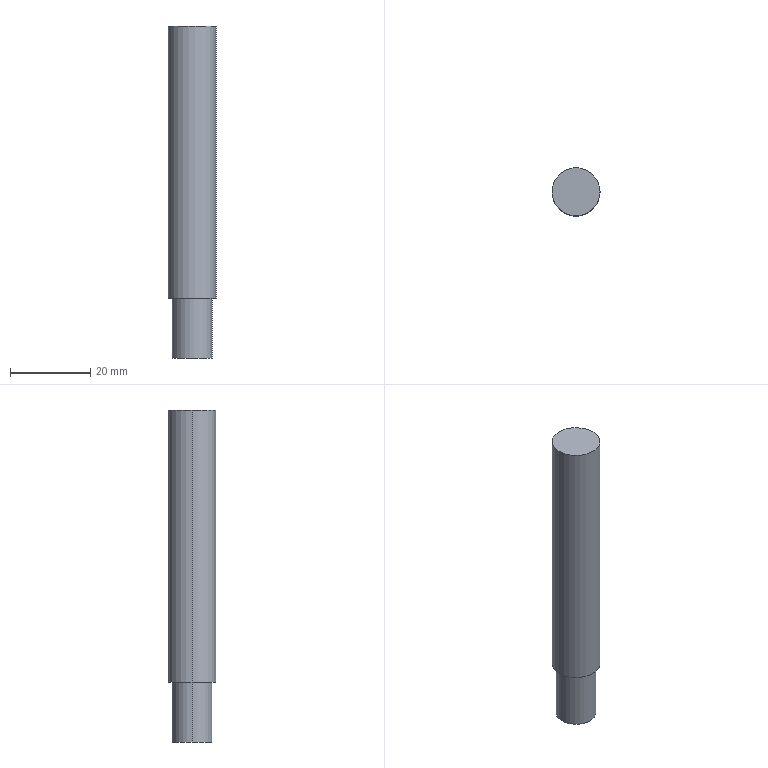Part | STEP file | 导柱-2 | 1 solid | 7 faces | box 12 x 12 x 83 mm | volume 8869 mm3 | cylinder 4 | plane 3 | commonest cylinder face diameters 10 x2 12 x2
STEP:
#1=CARTESIAN_POINT('',(-17.,43.,68.));
#2=VERTEX_POINT('',#1);
#3=CARTESIAN_POINT('',(-29.,43.,68.));
#4=VERTEX_POINT('',#3);
#5=CARTESIAN_POINT('',(-23.,43.,68.));
#6=DIRECTION('',(0.,0.,1.));
#7=DIRECTION('',(1.,0.,0.));
#8=AXIS2_PLACEMENT_3D('',#5,#6,#7);
#9=CIRCLE('',#8,6.);
#10=EDGE_CURVE('',#2,#4,#9,.T.);
#11=ORIENTED_EDGE('',*,*,#10,.F.);
#12=CARTESIAN_POINT('',(-17.,43.,0.));
#13=VERTEX_POINT('',#12);
#14=CARTESIAN_POINT('',(-17.,43.,68.));
#15=DIRECTION('',(0.,0.,-1.));
#16=VECTOR('',#15,1000.);
#17=LINE('',#14,#16);
#18=EDGE_CURVE('',#2,#13,#17,.T.);
#19=ORIENTED_EDGE('',*,*,#18,.T.);
#20=CARTESIAN_POINT('',(-29.,43.,0.));
#21=VERTEX_POINT('',#20);
#22=CARTESIAN_POINT('',(-23.,43.,0.));
#23=DIRECTION('',(0.,0.,1.));
#24=DIRECTION('',(1.,0.,0.));
#25=AXIS2_PLACEMENT_3D('',#22,#23,#24);
#26=CIRCLE('',#25,6.);
#27=EDGE_CURVE('',#13,#21,#26,.T.);
#28=ORIENTED_EDGE('',*,*,#27,.T.);
#29=CARTESIAN_POINT('',(-29.,43.,68.));
#30=DIRECTION('',(0.,0.,-1.));
#31=VECTOR('',#30,1000.);
#32=LINE('',#29,#31);
#33=EDGE_CURVE('',#4,#21,#32,.T.);
#34=ORIENTED_EDGE('',*,*,#33,.F.);
#35=EDGE_LOOP('',(#11,#19,#28,#34));
#36=FACE_OUTER_BOUND('',#35,.T.);
#37=CARTESIAN_POINT('',(-23.,43.,68.));
#38=DIRECTION('',(0.,0.,-1.));
#39=DIRECTION('',(-1.,0.,0.));
#40=AXIS2_PLACEMENT_3D('',#37,#38,#39);
#41=CYLINDRICAL_SURFACE('',#40,6.);
#42=ADVANCED_FACE('',(#36),#41,.T.);
#43=CARTESIAN_POINT('',(-18.,43.,-15.));
#44=VERTEX_POINT('',#43);
#45=CARTESIAN_POINT('',(-28.,43.,-15.));
#46=VERTEX_POINT('',#45);
#47=CARTESIAN_POINT('',(-23.,43.,-15.));
#48=DIRECTION('',(0.,0.,1.));
#49=DIRECTION('',(1.,0.,0.));
#50=AXIS2_PLACEMENT_3D('',#47,#48,#49);
#51=CIRCLE('',#50,5.);
#52=EDGE_CURVE('',#44,#46,#51,.T.);
#53=ORIENTED_EDGE('',*,*,#52,.T.);
#54=CARTESIAN_POINT('',(-28.,43.,0.));
#55=VERTEX_POINT('',#54);
#56=CARTESIAN_POINT('',(-28.,43.,-15.));
#57=DIRECTION('',(0.,0.,1.));
#58=VECTOR('',#57,1000.);
#59=LINE('',#56,#58);
#60=EDGE_CURVE('',#46,#55,#59,.T.);
#61=ORIENTED_EDGE('',*,*,#60,.T.);
#62=CARTESIAN_POINT('',(-18.,43.,0.));
#63=VERTEX_POINT('',#62);
#64=CARTESIAN_POINT('',(-23.,43.,0.));
#65=DIRECTION('',(0.,0.,1.));
#66=DIRECTION('',(1.,0.,0.));
#67=AXIS2_PLACEMENT_3D('',#64,#65,#66);
#68=CIRCLE('',#67,5.);
#69=EDGE_CURVE('',#63,#55,#68,.T.);
#70=ORIENTED_EDGE('',*,*,#69,.F.);
#71=CARTESIAN_POINT('',(-18.,43.,-15.));
#72=DIRECTION('',(0.,0.,1.));
#73=VECTOR('',#72,1000.);
#74=LINE('',#71,#73);
#75=EDGE_CURVE('',#44,#63,#74,.T.);
#76=ORIENTED_EDGE('',*,*,#75,.F.);
#77=EDGE_LOOP('',(#53,#61,#70,#76));
#78=FACE_OUTER_BOUND('',#77,.T.);
#79=CARTESIAN_POINT('',(-23.,43.,-15.));
#80=DIRECTION('',(0.,0.,1.));
#81=DIRECTION('',(1.,0.,0.));
#82=AXIS2_PLACEMENT_3D('',#79,#80,#81);
#83=CYLINDRICAL_SURFACE('',#82,5.);
#84=ADVANCED_FACE('',(#78),#83,.T.);
#85=ORIENTED_EDGE('',*,*,#60,.F.);
#86=CARTESIAN_POINT('',(-23.,43.,-15.));
#87=DIRECTION('',(0.,0.,1.));
#88=DIRECTION('',(1.,0.,0.));
#89=AXIS2_PLACEMENT_3D('',#86,#87,#88);
#90=CIRCLE('',#89,5.);
#91=EDGE_CURVE('',#46,#44,#90,.T.);
#92=ORIENTED_EDGE('',*,*,#91,.T.);
#93=ORIENTED_EDGE('',*,*,#75,.T.);
#94=CARTESIAN_POINT('',(-23.,43.,0.));
#95=DIRECTION('',(0.,0.,1.));
#96=DIRECTION('',(1.,0.,0.));
#97=AXIS2_PLACEMENT_3D('',#94,#95,#96);
#98=CIRCLE('',#97,5.);
#99=EDGE_CURVE('',#55,#63,#98,.T.);
#100=ORIENTED_EDGE('',*,*,#99,.F.);
#101=EDGE_LOOP('',(#85,#92,#93,#100));
#102=FACE_OUTER_BOUND('',#101,.T.);
#103=CARTESIAN_POINT('',(-23.,43.,-15.));
#104=DIRECTION('',(0.,0.,1.));
#105=DIRECTION('',(1.,0.,0.));
#106=AXIS2_PLACEMENT_3D('',#103,#104,#105);
#107=CYLINDRICAL_SURFACE('',#106,5.);
#108=ADVANCED_FACE('',(#102),#107,.T.);
#109=ORIENTED_EDGE('',*,*,#52,.F.);
#110=ORIENTED_EDGE('',*,*,#91,.F.);
#111=EDGE_LOOP('',(#109,#110));
#112=FACE_OUTER_BOUND('',#111,.T.);
#113=CARTESIAN_POINT('',(-23.,43.,-15.));
#114=DIRECTION('',(0.,0.,1.));
#115=DIRECTION('',(1.,0.,0.));
#116=AXIS2_PLACEMENT_3D('',#113,#114,#115);
#117=PLANE('',#116);
#118=ADVANCED_FACE('',(#112),#117,.F.);
#119=ORIENTED_EDGE('',*,*,#18,.F.);
#120=CARTESIAN_POINT('',(-23.,43.,68.));
#121=DIRECTION('',(0.,0.,1.));
#122=DIRECTION('',(1.,0.,0.));
#123=AXIS2_PLACEMENT_3D('',#120,#121,#122);
#124=CIRCLE('',#123,6.);
#125=EDGE_CURVE('',#4,#2,#124,.T.);
#126=ORIENTED_EDGE('',*,*,#125,.F.);
#127=ORIENTED_EDGE('',*,*,#33,.T.);
#128=CARTESIAN_POINT('',(-23.,43.,0.));
#129=DIRECTION('',(0.,0.,1.));
#130=DIRECTION('',(1.,0.,0.));
#131=AXIS2_PLACEMENT_3D('',#128,#129,#130);
#132=CIRCLE('',#131,6.);
#133=EDGE_CURVE('',#21,#13,#132,.T.);
#134=ORIENTED_EDGE('',*,*,#133,.T.);
#135=EDGE_LOOP('',(#119,#126,#127,#134));
#136=FACE_OUTER_BOUND('',#135,.T.);
#137=CARTESIAN_POINT('',(-23.,43.,68.));
#138=DIRECTION('',(0.,0.,-1.));
#139=DIRECTION('',(-1.,0.,0.));
#140=AXIS2_PLACEMENT_3D('',#137,#138,#139);
#141=CYLINDRICAL_SURFACE('',#140,6.);
#142=ADVANCED_FACE('',(#136),#141,.T.);
#143=ORIENTED_EDGE('',*,*,#125,.T.);
#144=ORIENTED_EDGE('',*,*,#10,.T.);
#145=EDGE_LOOP('',(#143,#144));
#146=FACE_OUTER_BOUND('',#145,.T.);
#147=CARTESIAN_POINT('',(-23.,43.,68.));
#148=DIRECTION('',(0.,0.,1.));
#149=DIRECTION('',(1.,0.,0.));
#150=AXIS2_PLACEMENT_3D('',#147,#148,#149);
#151=PLANE('',#150);
#152=ADVANCED_FACE('',(#146),#151,.T.);
#153=ORIENTED_EDGE('',*,*,#69,.T.);
#154=ORIENTED_EDGE('',*,*,#99,.T.);
#155=EDGE_LOOP('',(#153,#154));
#156=FACE_BOUND('',#155,.T.);
#157=ORIENTED_EDGE('',*,*,#133,.F.);
#158=ORIENTED_EDGE('',*,*,#27,.F.);
#159=EDGE_LOOP('',(#157,#158));
#160=FACE_OUTER_BOUND('',#159,.T.);
#161=CARTESIAN_POINT('',(-23.,43.,0.));
#162=DIRECTION('',(0.,0.,1.));
#163=DIRECTION('',(1.,0.,0.));
#164=AXIS2_PLACEMENT_3D('',#161,#162,#163);
#165=PLANE('',#164);
#166=ADVANCED_FACE('',(#156,#160),#165,.F.);
#167=CLOSED_SHELL('',(#42,#84,#108,#118,#142,#152,#166));
#168=MANIFOLD_SOLID_BREP('',#167);
#169=CARTESIAN_POINT('',(0.,0.,0.));
#170=DIRECTION('',(0.,0.,1.));
#171=DIRECTION('',(1.,0.,0.));
#172=AXIS2_PLACEMENT_3D('',#169,#170,#171);
#173=(LENGTH_UNIT()NAMED_UNIT(*)SI_UNIT(.MILLI.,.METRE.));
#174=UNCERTAINTY_MEASURE_WITH_UNIT(LENGTH_MEASURE(0.00001),#173,'','');
#175=(NAMED_UNIT(*)PLANE_ANGLE_UNIT()SI_UNIT($,.RADIAN.));
#176=(NAMED_UNIT(*)SI_UNIT($,.STERADIAN.)SOLID_ANGLE_UNIT());
#177=(GEOMETRIC_REPRESENTATION_CONTEXT(3)GLOBAL_UNCERTAINTY_ASSIGNED_CONTEXT((#174))GLOBAL_UNIT_ASSIGNED_CONTEXT((#173,#175,#176))REPRESENTATION_CONTEXT('',''));
#178=ADVANCED_BREP_SHAPE_REPRESENTATION('',(#168,#172),#177);